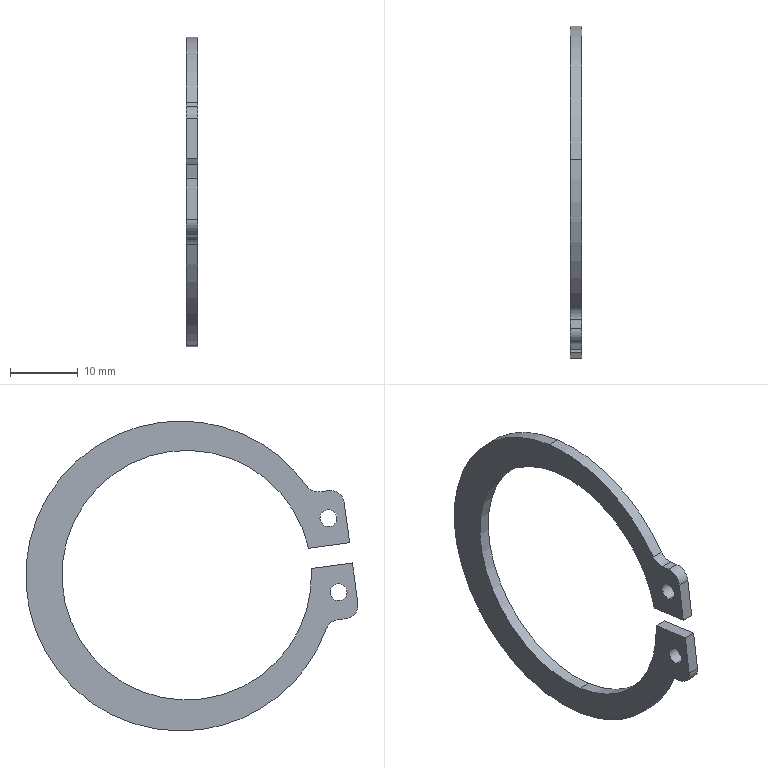Part | NX | features BREP 1 | 1 solid | 22 faces | box 1.75 x 48.899 x 45.6 mm | volume 1058 mm3 | cylinder 14 | plane 8 | commonest cylinder face diameters 2.5 x4 4 x4 36.73 x3 45.6 x3
STEP:
#1=CARTESIAN_POINT('',(-574.52,-22.174,-1.27));
#2=VERTEX_POINT('',#1);
#3=CARTESIAN_POINT('',(-574.52,-22.511,-3.747));
#4=VERTEX_POINT('',#3);
#5=CARTESIAN_POINT('',(-574.52,-22.343,-2.508));
#6=DIRECTION('',(1.,0.,0.));
#7=DIRECTION('',(0.,0.1349,0.9909));
#8=AXIS2_PLACEMENT_3D('',#5,#6,#7);
#9=CIRCLE('',#8,1.25);
#10=EDGE_CURVE('',#2,#4,#9,.T.);
#11=ORIENTED_EDGE('',*,*,#10,.T.);
#12=CARTESIAN_POINT('',(-576.27,-22.511,-3.747));
#13=VERTEX_POINT('',#12);
#14=CARTESIAN_POINT('',(-574.52,-22.511,-3.747));
#15=DIRECTION('',(-1.,0.,0.));
#16=VECTOR('',#15,1000.);
#17=LINE('',#14,#16);
#18=EDGE_CURVE('',#4,#13,#17,.T.);
#19=ORIENTED_EDGE('',*,*,#18,.T.);
#20=CARTESIAN_POINT('',(-576.27,-22.174,-1.27));
#21=VERTEX_POINT('',#20);
#22=CARTESIAN_POINT('',(-576.27,-22.343,-2.508));
#23=DIRECTION('',(1.,0.,0.));
#24=DIRECTION('',(0.,0.1349,0.9909));
#25=AXIS2_PLACEMENT_3D('',#22,#23,#24);
#26=CIRCLE('',#25,1.25);
#27=EDGE_CURVE('',#21,#13,#26,.T.);
#28=ORIENTED_EDGE('',*,*,#27,.F.);
#29=CARTESIAN_POINT('',(-574.52,-22.174,-1.27));
#30=DIRECTION('',(-1.,0.,0.));
#31=VECTOR('',#30,1000.);
#32=LINE('',#29,#31);
#33=EDGE_CURVE('',#2,#21,#32,.T.);
#34=ORIENTED_EDGE('',*,*,#33,.F.);
#35=EDGE_LOOP('',(#11,#19,#28,#34));
#36=FACE_BOUND('',#35,.T.);
#37=CARTESIAN_POINT('',(-574.52,-22.343,-2.508));
#38=DIRECTION('',(-1.,0.,0.));
#39=DIRECTION('',(0.,-0.1349,-0.9909));
#40=AXIS2_PLACEMENT_3D('',#37,#38,#39);
#41=CYLINDRICAL_SURFACE('',#40,1.25);
#42=ADVANCED_FACE('',(#36),#41,.F.);
#43=CARTESIAN_POINT('',(-574.52,-20.69,9.63));
#44=VERTEX_POINT('',#43);
#45=CARTESIAN_POINT('',(-574.52,-21.027,7.153));
#46=VERTEX_POINT('',#45);
#47=CARTESIAN_POINT('',(-574.52,-20.859,8.391));
#48=DIRECTION('',(1.,0.,0.));
#49=DIRECTION('',(0.,0.1349,0.9909));
#50=AXIS2_PLACEMENT_3D('',#47,#48,#49);
#51=CIRCLE('',#50,1.25);
#52=EDGE_CURVE('',#44,#46,#51,.T.);
#53=ORIENTED_EDGE('',*,*,#52,.T.);
#54=CARTESIAN_POINT('',(-576.27,-21.027,7.153));
#55=VERTEX_POINT('',#54);
#56=CARTESIAN_POINT('',(-574.52,-21.027,7.153));
#57=DIRECTION('',(-1.,0.,0.));
#58=VECTOR('',#57,1000.);
#59=LINE('',#56,#58);
#60=EDGE_CURVE('',#46,#55,#59,.T.);
#61=ORIENTED_EDGE('',*,*,#60,.T.);
#62=CARTESIAN_POINT('',(-576.27,-20.69,9.63));
#63=VERTEX_POINT('',#62);
#64=CARTESIAN_POINT('',(-576.27,-20.859,8.391));
#65=DIRECTION('',(1.,0.,0.));
#66=DIRECTION('',(0.,0.1349,0.9909));
#67=AXIS2_PLACEMENT_3D('',#64,#65,#66);
#68=CIRCLE('',#67,1.25);
#69=EDGE_CURVE('',#63,#55,#68,.T.);
#70=ORIENTED_EDGE('',*,*,#69,.F.);
#71=CARTESIAN_POINT('',(-574.52,-20.69,9.63));
#72=DIRECTION('',(-1.,0.,0.));
#73=VECTOR('',#72,1000.);
#74=LINE('',#71,#73);
#75=EDGE_CURVE('',#44,#63,#74,.T.);
#76=ORIENTED_EDGE('',*,*,#75,.F.);
#77=EDGE_LOOP('',(#53,#61,#70,#76));
#78=FACE_BOUND('',#77,.T.);
#79=CARTESIAN_POINT('',(-574.52,-20.859,8.391));
#80=DIRECTION('',(-1.,0.,0.));
#81=DIRECTION('',(0.,-0.1349,-0.9909));
#82=AXIS2_PLACEMENT_3D('',#79,#80,#81);
#83=CYLINDRICAL_SURFACE('',#82,1.25);
#84=ADVANCED_FACE('',(#78),#83,.F.);
#85=CARTESIAN_POINT('',(-574.52,-2.478,-18.197));
#86=VERTEX_POINT('',#85);
#87=CARTESIAN_POINT('',(-574.52,-18.339,0.9834));
#88=VERTEX_POINT('',#87);
#89=CARTESIAN_POINT('',(-574.52,0.,0.));
#90=DIRECTION('',(-1.,0.,0.));
#91=DIRECTION('',(0.,0.1349,0.9909));
#92=AXIS2_PLACEMENT_3D('',#89,#90,#91);
#93=CIRCLE('',#92,18.365);
#94=EDGE_CURVE('',#86,#88,#93,.T.);
#95=ORIENTED_EDGE('',*,*,#94,.F.);
#96=CARTESIAN_POINT('',(-576.27,-2.478,-18.197));
#97=VERTEX_POINT('',#96);
#98=CARTESIAN_POINT('',(-574.52,-2.478,-18.197));
#99=DIRECTION('',(-1.,0.,0.));
#100=VECTOR('',#99,1000.);
#101=LINE('',#98,#100);
#102=EDGE_CURVE('',#86,#97,#101,.T.);
#103=ORIENTED_EDGE('',*,*,#102,.T.);
#104=CARTESIAN_POINT('',(-576.27,-18.339,0.9834));
#105=VERTEX_POINT('',#104);
#106=CARTESIAN_POINT('',(-576.27,0.,0.));
#107=DIRECTION('',(-1.,0.,0.));
#108=DIRECTION('',(0.,0.1349,0.9909));
#109=AXIS2_PLACEMENT_3D('',#106,#107,#108);
#110=CIRCLE('',#109,18.365);
#111=EDGE_CURVE('',#97,#105,#110,.T.);
#112=ORIENTED_EDGE('',*,*,#111,.T.);
#113=CARTESIAN_POINT('',(-574.52,-18.339,0.9834));
#114=DIRECTION('',(-1.,0.,0.));
#115=VECTOR('',#114,1000.);
#116=LINE('',#113,#115);
#117=EDGE_CURVE('',#88,#105,#116,.T.);
#118=ORIENTED_EDGE('',*,*,#117,.F.);
#119=EDGE_LOOP('',(#95,#103,#112,#118));
#120=FACE_BOUND('',#119,.T.);
#121=CARTESIAN_POINT('',(-574.52,0.,0.));
#122=DIRECTION('',(-1.,0.,0.));
#123=DIRECTION('',(0.,-0.1349,-0.9909));
#124=AXIS2_PLACEMENT_3D('',#121,#122,#123);
#125=CYLINDRICAL_SURFACE('',#124,18.365);
#126=ADVANCED_FACE('',(#120),#125,.F.);
#127=ORIENTED_EDGE('',*,*,#102,.F.);
#128=CARTESIAN_POINT('',(-574.52,2.478,18.197));
#129=VERTEX_POINT('',#128);
#130=CARTESIAN_POINT('',(-574.52,0.,0.));
#131=DIRECTION('',(-1.,0.,0.));
#132=DIRECTION('',(0.,0.1349,0.9909));
#133=AXIS2_PLACEMENT_3D('',#130,#131,#132);
#134=CIRCLE('',#133,18.365);
#135=EDGE_CURVE('',#129,#86,#134,.T.);
#136=ORIENTED_EDGE('',*,*,#135,.F.);
#137=CARTESIAN_POINT('',(-576.27,2.478,18.197));
#138=VERTEX_POINT('',#137);
#139=CARTESIAN_POINT('',(-574.52,2.478,18.197));
#140=DIRECTION('',(-1.,0.,0.));
#141=VECTOR('',#140,1000.);
#142=LINE('',#139,#141);
#143=EDGE_CURVE('',#129,#138,#142,.T.);
#144=ORIENTED_EDGE('',*,*,#143,.T.);
#145=CARTESIAN_POINT('',(-576.27,0.,0.));
#146=DIRECTION('',(-1.,0.,0.));
#147=DIRECTION('',(0.,0.1349,0.9909));
#148=AXIS2_PLACEMENT_3D('',#145,#146,#147);
#149=CIRCLE('',#148,18.365);
#150=EDGE_CURVE('',#138,#97,#149,.T.);
#151=ORIENTED_EDGE('',*,*,#150,.T.);
#152=EDGE_LOOP('',(#127,#136,#144,#151));
#153=FACE_BOUND('',#152,.T.);
#154=CARTESIAN_POINT('',(-574.52,0.,0.));
#155=DIRECTION('',(-1.,0.,0.));
#156=DIRECTION('',(0.,-0.1349,-0.9909));
#157=AXIS2_PLACEMENT_3D('',#154,#155,#156);
#158=CYLINDRICAL_SURFACE('',#157,18.365);
#159=ADVANCED_FACE('',(#153),#158,.F.);
#160=CARTESIAN_POINT('',(-574.52,-2.185,-22.713));
#161=VERTEX_POINT('',#160);
#162=CARTESIAN_POINT('',(-574.52,3.968,22.47));
#163=VERTEX_POINT('',#162);
#164=CARTESIAN_POINT('',(-574.52,0.8918,-0.1214));
#165=DIRECTION('',(1.,0.,0.));
#166=DIRECTION('',(0.,-0.1349,-0.9909));
#167=AXIS2_PLACEMENT_3D('',#164,#165,#166);
#168=CIRCLE('',#167,22.8);
#169=EDGE_CURVE('',#161,#163,#168,.T.);
#170=ORIENTED_EDGE('',*,*,#169,.F.);
#171=CARTESIAN_POINT('',(-576.27,-2.185,-22.713));
#172=VERTEX_POINT('',#171);
#173=CARTESIAN_POINT('',(-574.52,-2.185,-22.713));
#174=DIRECTION('',(-1.,0.,0.));
#175=VECTOR('',#174,1000.);
#176=LINE('',#173,#175);
#177=EDGE_CURVE('',#161,#172,#176,.T.);
#178=ORIENTED_EDGE('',*,*,#177,.T.);
#179=CARTESIAN_POINT('',(-576.27,3.968,22.47));
#180=VERTEX_POINT('',#179);
#181=CARTESIAN_POINT('',(-576.27,0.8918,-0.1214));
#182=DIRECTION('',(1.,0.,0.));
#183=DIRECTION('',(0.,-0.1349,-0.9909));
#184=AXIS2_PLACEMENT_3D('',#181,#182,#183);
#185=CIRCLE('',#184,22.8);
#186=EDGE_CURVE('',#172,#180,#185,.T.);
#187=ORIENTED_EDGE('',*,*,#186,.T.);
#188=CARTESIAN_POINT('',(-574.52,3.968,22.47));
#189=DIRECTION('',(-1.,0.,0.));
#190=VECTOR('',#189,1000.);
#191=LINE('',#188,#190);
#192=EDGE_CURVE('',#163,#180,#191,.T.);
#193=ORIENTED_EDGE('',*,*,#192,.F.);
#194=EDGE_LOOP('',(#170,#178,#187,#193));
#195=FACE_BOUND('',#194,.T.);
#196=CARTESIAN_POINT('',(-574.52,0.8918,-0.1214));
#197=DIRECTION('',(-1.,0.,0.));
#198=DIRECTION('',(0.,-0.1349,-0.9909));
#199=AXIS2_PLACEMENT_3D('',#196,#197,#198);
#200=CYLINDRICAL_SURFACE('',#199,22.8);
#201=ADVANCED_FACE('',(#195),#200,.T.);
#202=CARTESIAN_POINT('',(-574.52,-17.697,13.08));
#203=VERTEX_POINT('',#202);
#204=CARTESIAN_POINT('',(-574.52,0.8918,-0.1214));
#205=DIRECTION('',(1.,0.,0.));
#206=DIRECTION('',(0.,-0.1349,-0.9909));
#207=AXIS2_PLACEMENT_3D('',#204,#205,#206);
#208=CIRCLE('',#207,22.8);
#209=EDGE_CURVE('',#163,#203,#208,.T.);
#210=ORIENTED_EDGE('',*,*,#209,.F.);
#211=ORIENTED_EDGE('',*,*,#192,.T.);
#212=CARTESIAN_POINT('',(-576.27,-17.697,13.08));
#213=VERTEX_POINT('',#212);
#214=CARTESIAN_POINT('',(-576.27,0.8918,-0.1214));
#215=DIRECTION('',(1.,0.,0.));
#216=DIRECTION('',(0.,-0.1349,-0.9909));
#217=AXIS2_PLACEMENT_3D('',#214,#215,#216);
#218=CIRCLE('',#217,22.8);
#219=EDGE_CURVE('',#180,#213,#218,.T.);
#220=ORIENTED_EDGE('',*,*,#219,.T.);
#221=CARTESIAN_POINT('',(-574.52,-17.697,13.08));
#222=DIRECTION('',(-1.,0.,0.));
#223=VECTOR('',#222,1000.);
#224=LINE('',#221,#223);
#225=EDGE_CURVE('',#203,#213,#224,.T.);
#226=ORIENTED_EDGE('',*,*,#225,.F.);
#227=EDGE_LOOP('',(#210,#211,#220,#226));
#228=FACE_BOUND('',#227,.T.);
#229=CARTESIAN_POINT('',(-574.52,0.8918,-0.1214));
#230=DIRECTION('',(-1.,0.,0.));
#231=DIRECTION('',(0.,-0.1349,-0.9909));
#232=AXIS2_PLACEMENT_3D('',#229,#230,#231);
#233=CYLINDRICAL_SURFACE('',#232,22.8);
#234=ADVANCED_FACE('',(#228),#233,.T.);
#235=ORIENTED_EDGE('',*,*,#52,.F.);
#236=CARTESIAN_POINT('',(-574.52,-20.859,8.391));
#237=DIRECTION('',(1.,0.,0.));
#238=DIRECTION('',(0.,0.1349,0.9909));
#239=AXIS2_PLACEMENT_3D('',#236,#237,#238);
#240=CIRCLE('',#239,1.25);
#241=EDGE_CURVE('',#46,#44,#240,.T.);
#242=ORIENTED_EDGE('',*,*,#241,.F.);
#243=EDGE_LOOP('',(#235,#242));
#244=FACE_BOUND('',#243,.T.);
#245=CARTESIAN_POINT('',(-574.52,-24.379,1.806));
#246=VERTEX_POINT('',#245);
#247=CARTESIAN_POINT('',(-574.52,-18.339,0.9834));
#248=DIRECTION('',(0.,-0.9909,0.1349));
#249=VECTOR('',#248,1000.);
#250=LINE('',#247,#249);
#251=EDGE_CURVE('',#88,#246,#250,.T.);
#252=ORIENTED_EDGE('',*,*,#251,.T.);
#253=CARTESIAN_POINT('',(-574.52,-25.189,-4.139));
#254=VERTEX_POINT('',#253);
#255=CARTESIAN_POINT('',(-574.52,-24.379,1.806));
#256=DIRECTION('',(0.,-0.1349,-0.9909));
#257=VECTOR('',#256,1000.);
#258=LINE('',#255,#257);
#259=EDGE_CURVE('',#246,#254,#258,.T.);
#260=ORIENTED_EDGE('',*,*,#259,.T.);
#261=CARTESIAN_POINT('',(-574.52,-23.477,-6.391));
#262=VERTEX_POINT('',#261);
#263=CARTESIAN_POINT('',(-574.52,-23.207,-4.409));
#264=DIRECTION('',(1.,0.,0.));
#265=DIRECTION('',(0.,-0.1349,-0.9909));
#266=AXIS2_PLACEMENT_3D('',#263,#264,#265);
#267=CIRCLE('',#266,2.);
#268=EDGE_CURVE('',#254,#262,#267,.T.);
#269=ORIENTED_EDGE('',*,*,#268,.T.);
#270=CARTESIAN_POINT('',(-574.52,-22.162,-6.57));
#271=VERTEX_POINT('',#270);
#272=CARTESIAN_POINT('',(-574.52,-23.477,-6.391));
#273=DIRECTION('',(0.,0.9909,-0.1349));
#274=VECTOR('',#273,1000.);
#275=LINE('',#272,#274);
#276=EDGE_CURVE('',#262,#271,#275,.T.);
#277=ORIENTED_EDGE('',*,*,#276,.T.);
#278=CARTESIAN_POINT('',(-574.52,-20.551,-7.872));
#279=VERTEX_POINT('',#278);
#280=CARTESIAN_POINT('',(-574.52,-22.431,-8.552));
#281=DIRECTION('',(-1.,0.,0.));
#282=DIRECTION('',(0.,0.1349,0.9909));
#283=AXIS2_PLACEMENT_3D('',#280,#281,#282);
#284=CIRCLE('',#283,2.);
#285=EDGE_CURVE('',#271,#279,#284,.T.);
#286=ORIENTED_EDGE('',*,*,#285,.T.);
#287=CARTESIAN_POINT('',(-574.52,0.8918,-0.1214));
#288=DIRECTION('',(1.,0.,0.));
#289=DIRECTION('',(0.,-0.1349,-0.9909));
#290=AXIS2_PLACEMENT_3D('',#287,#288,#289);
#291=CIRCLE('',#290,22.8);
#292=EDGE_CURVE('',#279,#161,#291,.T.);
#293=ORIENTED_EDGE('',*,*,#292,.T.);
#294=ORIENTED_EDGE('',*,*,#169,.T.);
#295=ORIENTED_EDGE('',*,*,#209,.T.);
#296=CARTESIAN_POINT('',(-574.52,-19.598,12.256));
#297=VERTEX_POINT('',#296);
#298=CARTESIAN_POINT('',(-574.52,-19.328,14.238));
#299=DIRECTION('',(-1.,0.,0.));
#300=DIRECTION('',(0.,0.1349,0.9909));
#301=AXIS2_PLACEMENT_3D('',#298,#299,#300);
#302=CIRCLE('',#301,2.);
#303=EDGE_CURVE('',#203,#297,#302,.T.);
#304=ORIENTED_EDGE('',*,*,#303,.T.);
#305=CARTESIAN_POINT('',(-574.52,-20.913,12.436));
#306=VERTEX_POINT('',#305);
#307=CARTESIAN_POINT('',(-574.52,-19.598,12.256));
#308=DIRECTION('',(0.,-0.9909,0.1349));
#309=VECTOR('',#308,1000.);
#310=LINE('',#307,#309);
#311=EDGE_CURVE('',#297,#306,#310,.T.);
#312=ORIENTED_EDGE('',*,*,#311,.T.);
#313=CARTESIAN_POINT('',(-574.52,-23.165,10.724));
#314=VERTEX_POINT('',#313);
#315=CARTESIAN_POINT('',(-574.52,-21.183,10.454));
#316=DIRECTION('',(1.,0.,0.));
#317=DIRECTION('',(0.,-0.1349,-0.9909));
#318=AXIS2_PLACEMENT_3D('',#315,#316,#317);
#319=CIRCLE('',#318,2.);
#320=EDGE_CURVE('',#306,#314,#319,.T.);
#321=ORIENTED_EDGE('',*,*,#320,.T.);
#322=CARTESIAN_POINT('',(-574.52,-23.974,4.779));
#323=VERTEX_POINT('',#322);
#324=CARTESIAN_POINT('',(-574.52,-23.165,10.724));
#325=DIRECTION('',(0.,-0.1349,-0.9909));
#326=VECTOR('',#325,1000.);
#327=LINE('',#324,#326);
#328=EDGE_CURVE('',#314,#323,#327,.T.);
#329=ORIENTED_EDGE('',*,*,#328,.T.);
#330=CARTESIAN_POINT('',(-574.52,-17.934,3.956));
#331=VERTEX_POINT('',#330);
#332=CARTESIAN_POINT('',(-574.52,-23.974,4.779));
#333=DIRECTION('',(0.,0.9909,-0.1349));
#334=VECTOR('',#333,1000.);
#335=LINE('',#332,#334);
#336=EDGE_CURVE('',#323,#331,#335,.T.);
#337=ORIENTED_EDGE('',*,*,#336,.T.);
#338=CARTESIAN_POINT('',(-574.52,0.,0.));
#339=DIRECTION('',(-1.,0.,0.));
#340=DIRECTION('',(0.,0.1349,0.9909));
#341=AXIS2_PLACEMENT_3D('',#338,#339,#340);
#342=CIRCLE('',#341,18.365);
#343=EDGE_CURVE('',#331,#129,#342,.T.);
#344=ORIENTED_EDGE('',*,*,#343,.T.);
#345=ORIENTED_EDGE('',*,*,#135,.T.);
#346=ORIENTED_EDGE('',*,*,#94,.T.);
#347=EDGE_LOOP('',(#252,#260,#269,#277,#286,#293,#294,#295,#304,#312,#321,#329,#337,#344,#345,#346));
#348=FACE_BOUND('',#347,.T.);
#349=ORIENTED_EDGE('',*,*,#10,.F.);
#350=CARTESIAN_POINT('',(-574.52,-22.343,-2.508));
#351=DIRECTION('',(1.,0.,0.));
#352=DIRECTION('',(0.,0.1349,0.9909));
#353=AXIS2_PLACEMENT_3D('',#350,#351,#352);
#354=CIRCLE('',#353,1.25);
#355=EDGE_CURVE('',#4,#2,#354,.T.);
#356=ORIENTED_EDGE('',*,*,#355,.F.);
#357=EDGE_LOOP('',(#349,#356));
#358=FACE_BOUND('',#357,.T.);
#359=CARTESIAN_POINT('',(-574.52,-23.207,-4.409));
#360=DIRECTION('',(1.,0.,0.));
#361=DIRECTION('',(0.,0.1349,0.9909));
#362=AXIS2_PLACEMENT_3D('',#359,#360,#361);
#363=PLANE('',#362);
#364=ADVANCED_FACE('',(#244,#348,#358),#363,.T.);
#365=CARTESIAN_POINT('',(-576.27,-24.379,1.806));
#366=VERTEX_POINT('',#365);
#367=CARTESIAN_POINT('',(-576.27,-18.339,0.9834));
#368=DIRECTION('',(0.,-0.9909,0.1349));
#369=VECTOR('',#368,1000.);
#370=LINE('',#367,#369);
#371=EDGE_CURVE('',#105,#366,#370,.T.);
#372=ORIENTED_EDGE('',*,*,#371,.F.);
#373=ORIENTED_EDGE('',*,*,#111,.F.);
#374=ORIENTED_EDGE('',*,*,#150,.F.);
#375=CARTESIAN_POINT('',(-576.27,-17.934,3.956));
#376=VERTEX_POINT('',#375);
#377=CARTESIAN_POINT('',(-576.27,0.,0.));
#378=DIRECTION('',(-1.,0.,0.));
#379=DIRECTION('',(0.,0.1349,0.9909));
#380=AXIS2_PLACEMENT_3D('',#377,#378,#379);
#381=CIRCLE('',#380,18.365);
#382=EDGE_CURVE('',#376,#138,#381,.T.);
#383=ORIENTED_EDGE('',*,*,#382,.F.);
#384=CARTESIAN_POINT('',(-576.27,-23.974,4.779));
#385=VERTEX_POINT('',#384);
#386=CARTESIAN_POINT('',(-576.27,-23.974,4.779));
#387=DIRECTION('',(0.,0.9909,-0.1349));
#388=VECTOR('',#387,1000.);
#389=LINE('',#386,#388);
#390=EDGE_CURVE('',#385,#376,#389,.T.);
#391=ORIENTED_EDGE('',*,*,#390,.F.);
#392=CARTESIAN_POINT('',(-576.27,-23.165,10.724));
#393=VERTEX_POINT('',#392);
#394=CARTESIAN_POINT('',(-576.27,-23.165,10.724));
#395=DIRECTION('',(0.,-0.1349,-0.9909));
#396=VECTOR('',#395,1000.);
#397=LINE('',#394,#396);
#398=EDGE_CURVE('',#393,#385,#397,.T.);
#399=ORIENTED_EDGE('',*,*,#398,.F.);
#400=CARTESIAN_POINT('',(-576.27,-20.913,12.436));
#401=VERTEX_POINT('',#400);
#402=CARTESIAN_POINT('',(-576.27,-21.183,10.454));
#403=DIRECTION('',(1.,0.,0.));
#404=DIRECTION('',(0.,-0.1349,-0.9909));
#405=AXIS2_PLACEMENT_3D('',#402,#403,#404);
#406=CIRCLE('',#405,2.);
#407=EDGE_CURVE('',#401,#393,#406,.T.);
#408=ORIENTED_EDGE('',*,*,#407,.F.);
#409=CARTESIAN_POINT('',(-576.27,-19.598,12.256));
#410=VERTEX_POINT('',#409);
#411=CARTESIAN_POINT('',(-576.27,-19.598,12.256));
#412=DIRECTION('',(0.,-0.9909,0.1349));
#413=VECTOR('',#412,1000.);
#414=LINE('',#411,#413);
#415=EDGE_CURVE('',#410,#401,#414,.T.);
#416=ORIENTED_EDGE('',*,*,#415,.F.);
#417=CARTESIAN_POINT('',(-576.27,-19.328,14.238));
#418=DIRECTION('',(-1.,0.,0.));
#419=DIRECTION('',(0.,0.1349,0.9909));
#420=AXIS2_PLACEMENT_3D('',#417,#418,#419);
#421=CIRCLE('',#420,2.);
#422=EDGE_CURVE('',#213,#410,#421,.T.);
#423=ORIENTED_EDGE('',*,*,#422,.F.);
#424=ORIENTED_EDGE('',*,*,#219,.F.);
#425=ORIENTED_EDGE('',*,*,#186,.F.);
#426=CARTESIAN_POINT('',(-576.27,-20.551,-7.872));
#427=VERTEX_POINT('',#426);
#428=CARTESIAN_POINT('',(-576.27,0.8918,-0.1214));
#429=DIRECTION('',(1.,0.,0.));
#430=DIRECTION('',(0.,-0.1349,-0.9909));
#431=AXIS2_PLACEMENT_3D('',#428,#429,#430);
#432=CIRCLE('',#431,22.8);
#433=EDGE_CURVE('',#427,#172,#432,.T.);
#434=ORIENTED_EDGE('',*,*,#433,.F.);
#435=CARTESIAN_POINT('',(-576.27,-22.162,-6.57));
#436=VERTEX_POINT('',#435);
#437=CARTESIAN_POINT('',(-576.27,-22.431,-8.552));
#438=DIRECTION('',(-1.,0.,0.));
#439=DIRECTION('',(0.,0.1349,0.9909));
#440=AXIS2_PLACEMENT_3D('',#437,#438,#439);
#441=CIRCLE('',#440,2.);
#442=EDGE_CURVE('',#436,#427,#441,.T.);
#443=ORIENTED_EDGE('',*,*,#442,.F.);
#444=CARTESIAN_POINT('',(-576.27,-23.477,-6.391));
#445=VERTEX_POINT('',#444);
#446=CARTESIAN_POINT('',(-576.27,-23.477,-6.391));
#447=DIRECTION('',(0.,0.9909,-0.1349));
#448=VECTOR('',#447,1000.);
#449=LINE('',#446,#448);
#450=EDGE_CURVE('',#445,#436,#449,.T.);
#451=ORIENTED_EDGE('',*,*,#450,.F.);
#452=CARTESIAN_POINT('',(-576.27,-25.189,-4.139));
#453=VERTEX_POINT('',#452);
#454=CARTESIAN_POINT('',(-576.27,-23.207,-4.409));
#455=DIRECTION('',(1.,0.,0.));
#456=DIRECTION('',(0.,-0.1349,-0.9909));
#457=AXIS2_PLACEMENT_3D('',#454,#455,#456);
#458=CIRCLE('',#457,2.);
#459=EDGE_CURVE('',#453,#445,#458,.T.);
#460=ORIENTED_EDGE('',*,*,#459,.F.);
#461=CARTESIAN_POINT('',(-576.27,-24.379,1.806));
#462=DIRECTION('',(0.,-0.1349,-0.9909));
#463=VECTOR('',#462,1000.);
#464=LINE('',#461,#463);
#465=EDGE_CURVE('',#366,#453,#464,.T.);
#466=ORIENTED_EDGE('',*,*,#465,.F.);
#467=EDGE_LOOP('',(#372,#373,#374,#383,#391,#399,#408,#416,#423,#424,#425,#434,#443,#451,#460,#466));
#468=FACE_BOUND('',#467,.T.);
#469=ORIENTED_EDGE('',*,*,#69,.T.);
#470=CARTESIAN_POINT('',(-576.27,-20.859,8.391));
#471=DIRECTION('',(1.,0.,0.));
#472=DIRECTION('',(0.,0.1349,0.9909));
#473=AXIS2_PLACEMENT_3D('',#470,#471,#472);
#474=CIRCLE('',#473,1.25);
#475=EDGE_CURVE('',#55,#63,#474,.T.);
#476=ORIENTED_EDGE('',*,*,#475,.T.);
#477=EDGE_LOOP('',(#469,#476));
#478=FACE_BOUND('',#477,.T.);
#479=ORIENTED_EDGE('',*,*,#27,.T.);
#480=CARTESIAN_POINT('',(-576.27,-22.343,-2.508));
#481=DIRECTION('',(1.,0.,0.));
#482=DIRECTION('',(0.,0.1349,0.9909));
#483=AXIS2_PLACEMENT_3D('',#480,#481,#482);
#484=CIRCLE('',#483,1.25);
#485=EDGE_CURVE('',#13,#21,#484,.T.);
#486=ORIENTED_EDGE('',*,*,#485,.T.);
#487=EDGE_LOOP('',(#479,#486));
#488=FACE_BOUND('',#487,.T.);
#489=CARTESIAN_POINT('',(-576.27,-23.207,-4.409));
#490=DIRECTION('',(1.,0.,0.));
#491=DIRECTION('',(0.,0.1349,0.9909));
#492=AXIS2_PLACEMENT_3D('',#489,#490,#491);
#493=PLANE('',#492);
#494=ADVANCED_FACE('',(#468,#478,#488),#493,.F.);
#495=ORIENTED_EDGE('',*,*,#371,.T.);
#496=CARTESIAN_POINT('',(-574.52,-24.379,1.806));
#497=DIRECTION('',(-1.,0.,0.));
#498=VECTOR('',#497,1000.);
#499=LINE('',#496,#498);
#500=EDGE_CURVE('',#246,#366,#499,.T.);
#501=ORIENTED_EDGE('',*,*,#500,.F.);
#502=ORIENTED_EDGE('',*,*,#251,.F.);
#503=ORIENTED_EDGE('',*,*,#117,.T.);
#504=EDGE_LOOP('',(#495,#501,#502,#503));
#505=FACE_BOUND('',#504,.T.);
#506=CARTESIAN_POINT('',(-574.52,-18.339,0.9834));
#507=DIRECTION('',(0.,-0.1349,-0.9909));
#508=DIRECTION('',(0.,-0.9909,0.1349));
#509=AXIS2_PLACEMENT_3D('',#506,#507,#508);
#510=PLANE('',#509);
#511=ADVANCED_FACE('',(#505),#510,.F.);
#512=ORIENTED_EDGE('',*,*,#465,.T.);
#513=CARTESIAN_POINT('',(-574.52,-25.189,-4.139));
#514=DIRECTION('',(-1.,0.,0.));
#515=VECTOR('',#514,1000.);
#516=LINE('',#513,#515);
#517=EDGE_CURVE('',#254,#453,#516,.T.);
#518=ORIENTED_EDGE('',*,*,#517,.F.);
#519=ORIENTED_EDGE('',*,*,#259,.F.);
#520=ORIENTED_EDGE('',*,*,#500,.T.);
#521=EDGE_LOOP('',(#512,#518,#519,#520));
#522=FACE_BOUND('',#521,.T.);
#523=CARTESIAN_POINT('',(-574.52,-24.379,1.806));
#524=DIRECTION('',(0.,0.9909,-0.1349));
#525=DIRECTION('',(0.,-0.1349,-0.9909));
#526=AXIS2_PLACEMENT_3D('',#523,#524,#525);
#527=PLANE('',#526);
#528=ADVANCED_FACE('',(#522),#527,.F.);
#529=ORIENTED_EDGE('',*,*,#459,.T.);
#530=CARTESIAN_POINT('',(-574.52,-23.477,-6.391));
#531=DIRECTION('',(-1.,0.,0.));
#532=VECTOR('',#531,1000.);
#533=LINE('',#530,#532);
#534=EDGE_CURVE('',#262,#445,#533,.T.);
#535=ORIENTED_EDGE('',*,*,#534,.F.);
#536=ORIENTED_EDGE('',*,*,#268,.F.);
#537=ORIENTED_EDGE('',*,*,#517,.T.);
#538=EDGE_LOOP('',(#529,#535,#536,#537));
#539=FACE_BOUND('',#538,.T.);
#540=CARTESIAN_POINT('',(-574.52,-23.207,-4.409));
#541=DIRECTION('',(-1.,0.,0.));
#542=DIRECTION('',(0.,-0.1349,-0.9909));
#543=AXIS2_PLACEMENT_3D('',#540,#541,#542);
#544=CYLINDRICAL_SURFACE('',#543,2.);
#545=ADVANCED_FACE('',(#539),#544,.T.);
#546=ORIENTED_EDGE('',*,*,#450,.T.);
#547=CARTESIAN_POINT('',(-574.52,-22.162,-6.57));
#548=DIRECTION('',(-1.,0.,0.));
#549=VECTOR('',#548,1000.);
#550=LINE('',#547,#549);
#551=EDGE_CURVE('',#271,#436,#550,.T.);
#552=ORIENTED_EDGE('',*,*,#551,.F.);
#553=ORIENTED_EDGE('',*,*,#276,.F.);
#554=ORIENTED_EDGE('',*,*,#534,.T.);
#555=EDGE_LOOP('',(#546,#552,#553,#554));
#556=FACE_BOUND('',#555,.T.);
#557=CARTESIAN_POINT('',(-574.52,-23.477,-6.391));
#558=DIRECTION('',(0.,0.1349,0.9909));
#559=DIRECTION('',(0.,0.9909,-0.1349));
#560=AXIS2_PLACEMENT_3D('',#557,#558,#559);
#561=PLANE('',#560);
#562=ADVANCED_FACE('',(#556),#561,.F.);
#563=ORIENTED_EDGE('',*,*,#442,.T.);
#564=CARTESIAN_POINT('',(-574.52,-20.551,-7.872));
#565=DIRECTION('',(-1.,0.,0.));
#566=VECTOR('',#565,1000.);
#567=LINE('',#564,#566);
#568=EDGE_CURVE('',#279,#427,#567,.T.);
#569=ORIENTED_EDGE('',*,*,#568,.F.);
#570=ORIENTED_EDGE('',*,*,#285,.F.);
#571=ORIENTED_EDGE('',*,*,#551,.T.);
#572=EDGE_LOOP('',(#563,#569,#570,#571));
#573=FACE_BOUND('',#572,.T.);
#574=CARTESIAN_POINT('',(-574.52,-22.431,-8.552));
#575=DIRECTION('',(-1.,0.,0.));
#576=DIRECTION('',(0.,-0.1349,-0.9909));
#577=AXIS2_PLACEMENT_3D('',#574,#575,#576);
#578=CYLINDRICAL_SURFACE('',#577,2.);
#579=ADVANCED_FACE('',(#573),#578,.F.);
#580=ORIENTED_EDGE('',*,*,#177,.F.);
#581=ORIENTED_EDGE('',*,*,#292,.F.);
#582=ORIENTED_EDGE('',*,*,#568,.T.);
#583=ORIENTED_EDGE('',*,*,#433,.T.);
#584=EDGE_LOOP('',(#580,#581,#582,#583));
#585=FACE_BOUND('',#584,.T.);
#586=CARTESIAN_POINT('',(-574.52,0.8918,-0.1214));
#587=DIRECTION('',(-1.,0.,0.));
#588=DIRECTION('',(0.,-0.1349,-0.9909));
#589=AXIS2_PLACEMENT_3D('',#586,#587,#588);
#590=CYLINDRICAL_SURFACE('',#589,22.8);
#591=ADVANCED_FACE('',(#585),#590,.T.);
#592=ORIENTED_EDGE('',*,*,#422,.T.);
#593=CARTESIAN_POINT('',(-574.52,-19.598,12.256));
#594=DIRECTION('',(-1.,0.,0.));
#595=VECTOR('',#594,1000.);
#596=LINE('',#593,#595);
#597=EDGE_CURVE('',#297,#410,#596,.T.);
#598=ORIENTED_EDGE('',*,*,#597,.F.);
#599=ORIENTED_EDGE('',*,*,#303,.F.);
#600=ORIENTED_EDGE('',*,*,#225,.T.);
#601=EDGE_LOOP('',(#592,#598,#599,#600));
#602=FACE_BOUND('',#601,.T.);
#603=CARTESIAN_POINT('',(-574.52,-19.328,14.238));
#604=DIRECTION('',(-1.,0.,0.));
#605=DIRECTION('',(0.,-0.1349,-0.9909));
#606=AXIS2_PLACEMENT_3D('',#603,#604,#605);
#607=CYLINDRICAL_SURFACE('',#606,2.);
#608=ADVANCED_FACE('',(#602),#607,.F.);
#609=ORIENTED_EDGE('',*,*,#415,.T.);
#610=CARTESIAN_POINT('',(-574.52,-20.913,12.436));
#611=DIRECTION('',(-1.,0.,0.));
#612=VECTOR('',#611,1000.);
#613=LINE('',#610,#612);
#614=EDGE_CURVE('',#306,#401,#613,.T.);
#615=ORIENTED_EDGE('',*,*,#614,.F.);
#616=ORIENTED_EDGE('',*,*,#311,.F.);
#617=ORIENTED_EDGE('',*,*,#597,.T.);
#618=EDGE_LOOP('',(#609,#615,#616,#617));
#619=FACE_BOUND('',#618,.T.);
#620=CARTESIAN_POINT('',(-574.52,-19.598,12.256));
#621=DIRECTION('',(0.,-0.1349,-0.9909));
#622=DIRECTION('',(1.,0.,0.));
#623=AXIS2_PLACEMENT_3D('',#620,#621,#622);
#624=PLANE('',#623);
#625=ADVANCED_FACE('',(#619),#624,.F.);
#626=ORIENTED_EDGE('',*,*,#407,.T.);
#627=CARTESIAN_POINT('',(-574.52,-23.165,10.724));
#628=DIRECTION('',(-1.,0.,0.));
#629=VECTOR('',#628,1000.);
#630=LINE('',#627,#629);
#631=EDGE_CURVE('',#314,#393,#630,.T.);
#632=ORIENTED_EDGE('',*,*,#631,.F.);
#633=ORIENTED_EDGE('',*,*,#320,.F.);
#634=ORIENTED_EDGE('',*,*,#614,.T.);
#635=EDGE_LOOP('',(#626,#632,#633,#634));
#636=FACE_BOUND('',#635,.T.);
#637=CARTESIAN_POINT('',(-574.52,-21.183,10.454));
#638=DIRECTION('',(-1.,0.,0.));
#639=DIRECTION('',(0.,-0.1349,-0.9909));
#640=AXIS2_PLACEMENT_3D('',#637,#638,#639);
#641=CYLINDRICAL_SURFACE('',#640,2.);
#642=ADVANCED_FACE('',(#636),#641,.T.);
#643=ORIENTED_EDGE('',*,*,#398,.T.);
#644=CARTESIAN_POINT('',(-574.52,-23.974,4.779));
#645=DIRECTION('',(-1.,0.,0.));
#646=VECTOR('',#645,1000.);
#647=LINE('',#644,#646);
#648=EDGE_CURVE('',#323,#385,#647,.T.);
#649=ORIENTED_EDGE('',*,*,#648,.F.);
#650=ORIENTED_EDGE('',*,*,#328,.F.);
#651=ORIENTED_EDGE('',*,*,#631,.T.);
#652=EDGE_LOOP('',(#643,#649,#650,#651));
#653=FACE_BOUND('',#652,.T.);
#654=CARTESIAN_POINT('',(-574.52,-23.165,10.724));
#655=DIRECTION('',(0.,0.9909,-0.1349));
#656=DIRECTION('',(0.,-0.1349,-0.9909));
#657=AXIS2_PLACEMENT_3D('',#654,#655,#656);
#658=PLANE('',#657);
#659=ADVANCED_FACE('',(#653),#658,.F.);
#660=ORIENTED_EDGE('',*,*,#390,.T.);
#661=CARTESIAN_POINT('',(-574.52,-17.934,3.956));
#662=DIRECTION('',(-1.,0.,0.));
#663=VECTOR('',#662,1000.);
#664=LINE('',#661,#663);
#665=EDGE_CURVE('',#331,#376,#664,.T.);
#666=ORIENTED_EDGE('',*,*,#665,.F.);
#667=ORIENTED_EDGE('',*,*,#336,.F.);
#668=ORIENTED_EDGE('',*,*,#648,.T.);
#669=EDGE_LOOP('',(#660,#666,#667,#668));
#670=FACE_BOUND('',#669,.T.);
#671=CARTESIAN_POINT('',(-574.52,-23.974,4.779));
#672=DIRECTION('',(0.,0.1349,0.9909));
#673=DIRECTION('',(0.,0.9909,-0.1349));
#674=AXIS2_PLACEMENT_3D('',#671,#672,#673);
#675=PLANE('',#674);
#676=ADVANCED_FACE('',(#670),#675,.F.);
#677=ORIENTED_EDGE('',*,*,#143,.F.);
#678=ORIENTED_EDGE('',*,*,#343,.F.);
#679=ORIENTED_EDGE('',*,*,#665,.T.);
#680=ORIENTED_EDGE('',*,*,#382,.T.);
#681=EDGE_LOOP('',(#677,#678,#679,#680));
#682=FACE_BOUND('',#681,.T.);
#683=CARTESIAN_POINT('',(-574.52,0.,0.));
#684=DIRECTION('',(-1.,0.,0.));
#685=DIRECTION('',(0.,-0.1349,-0.9909));
#686=AXIS2_PLACEMENT_3D('',#683,#684,#685);
#687=CYLINDRICAL_SURFACE('',#686,18.365);
#688=ADVANCED_FACE('',(#682),#687,.F.);
#689=ORIENTED_EDGE('',*,*,#60,.F.);
#690=ORIENTED_EDGE('',*,*,#241,.T.);
#691=ORIENTED_EDGE('',*,*,#75,.T.);
#692=ORIENTED_EDGE('',*,*,#475,.F.);
#693=EDGE_LOOP('',(#689,#690,#691,#692));
#694=FACE_BOUND('',#693,.T.);
#695=CARTESIAN_POINT('',(-574.52,-20.859,8.391));
#696=DIRECTION('',(-1.,0.,0.));
#697=DIRECTION('',(0.,-0.1349,-0.9909));
#698=AXIS2_PLACEMENT_3D('',#695,#696,#697);
#699=CYLINDRICAL_SURFACE('',#698,1.25);
#700=ADVANCED_FACE('',(#694),#699,.F.);
#701=ORIENTED_EDGE('',*,*,#18,.F.);
#702=ORIENTED_EDGE('',*,*,#355,.T.);
#703=ORIENTED_EDGE('',*,*,#33,.T.);
#704=ORIENTED_EDGE('',*,*,#485,.F.);
#705=EDGE_LOOP('',(#701,#702,#703,#704));
#706=FACE_BOUND('',#705,.T.);
#707=CARTESIAN_POINT('',(-574.52,-22.343,-2.508));
#708=DIRECTION('',(-1.,0.,0.));
#709=DIRECTION('',(0.,-0.1349,-0.9909));
#710=AXIS2_PLACEMENT_3D('',#707,#708,#709);
#711=CYLINDRICAL_SURFACE('',#710,1.25);
#712=ADVANCED_FACE('',(#706),#711,.F.);
#713=CLOSED_SHELL('',(#42,#84,#126,#159,#201,#234,#364,#494,#511,#528,#545,#562,#579,#591,#608,#625,#642,#659,#676,#688,#700,#712));
#714=MANIFOLD_SOLID_BREP('',#713);
#715=(LENGTH_UNIT()NAMED_UNIT(*)SI_UNIT(.MILLI.,.METRE.));
#716=UNCERTAINTY_MEASURE_WITH_UNIT(LENGTH_MEASURE(0.00001),#715,'','');
#717=(NAMED_UNIT(*)PLANE_ANGLE_UNIT()SI_UNIT($,.RADIAN.));
#718=(NAMED_UNIT(*)SI_UNIT($,.STERADIAN.)SOLID_ANGLE_UNIT());
#719=(GEOMETRIC_REPRESENTATION_CONTEXT(3)GLOBAL_UNCERTAINTY_ASSIGNED_CONTEXT((#716))GLOBAL_UNIT_ASSIGNED_CONTEXT((#715,#717,#718))REPRESENTATION_CONTEXT('',''));
#720=ADVANCED_BREP_SHAPE_REPRESENTATION('',(#714),#719);